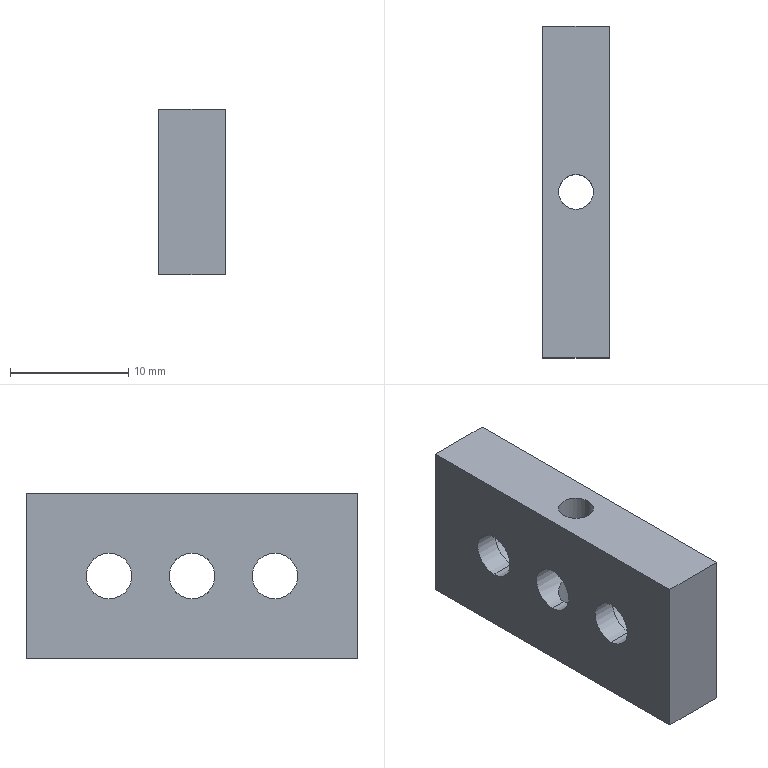Part | SolidWorks | features SplitBody 1 | 1 solid | 22 faces | box 5.6 x 28 x 14 mm | volume 1741 mm3 | cylinder 14 | plane 8 | commonest cylinder face diameters 3.85 x6 2.94 x4 7 x4
STEP:
#1=CARTESIAN_POINT('',(475.805,242.859,-463.116));
#2=VERTEX_POINT('',#1);
#3=CARTESIAN_POINT('',(478.745,242.859,-463.116));
#4=VERTEX_POINT('',#3);
#5=CARTESIAN_POINT('',(477.275,242.859,-463.116));
#6=DIRECTION('',(0.,0.,1.));
#7=DIRECTION('',(1.,0.,0.));
#8=AXIS2_PLACEMENT_3D('',#5,#6,#7);
#9=CIRCLE('',#8,1.47);
#10=EDGE_CURVE('',#2,#4,#9,.T.);
#11=ORIENTED_EDGE('',*,*,#10,.F.);
#12=CARTESIAN_POINT('',(475.805,242.859,-458.041));
#13=VERTEX_POINT('',#12);
#14=CARTESIAN_POINT('',(475.805,242.859,-449.116));
#15=DIRECTION('',(0.,0.,1.));
#16=VECTOR('',#15,1000.);
#17=LINE('',#14,#16);
#18=EDGE_CURVE('',#2,#13,#17,.T.);
#19=ORIENTED_EDGE('',*,*,#18,.T.);
#20=CARTESIAN_POINT('',(478.745,242.859,-458.041));
#21=VERTEX_POINT('',#20);
#22=CARTESIAN_POINT('',(478.745,242.859,-458.041));
#23=CARTESIAN_POINT('',(478.745,242.657,-458.041));
#24=CARTESIAN_POINT('',(478.702,242.455,-458.007));
#25=CARTESIAN_POINT('',(478.548,242.098,-457.894));
#26=CARTESIAN_POINT('',(478.439,241.942,-457.815));
#27=CARTESIAN_POINT('',(478.177,241.683,-457.648));
#28=CARTESIAN_POINT('',(478.024,241.58,-457.558));
#29=CARTESIAN_POINT('',(477.764,241.47,-457.449));
#30=CARTESIAN_POINT('',(477.671,241.44,-457.416));
#31=CARTESIAN_POINT('',(477.478,241.4,-457.371));
#32=CARTESIAN_POINT('',(477.376,241.389,-457.358));
#33=CARTESIAN_POINT('',(477.174,241.389,-457.359));
#34=CARTESIAN_POINT('',(477.072,241.4,-457.371));
#35=CARTESIAN_POINT('',(476.879,241.44,-457.417));
#36=CARTESIAN_POINT('',(476.788,241.469,-457.448));
#37=CARTESIAN_POINT('',(476.526,241.58,-457.558));
#38=CARTESIAN_POINT('',(476.375,241.682,-457.647));
#39=CARTESIAN_POINT('',(476.111,241.943,-457.816));
#40=CARTESIAN_POINT('',(476.004,242.096,-457.893));
#41=CARTESIAN_POINT('',(475.887,242.365,-457.979));
#42=CARTESIAN_POINT('',(475.857,242.459,-458.001));
#43=CARTESIAN_POINT('',(475.816,242.655,-458.032));
#44=CARTESIAN_POINT('',(475.805,242.757,-458.041));
#45=CARTESIAN_POINT('',(475.805,242.859,-458.041));
#46=B_SPLINE_CURVE_WITH_KNOTS('',3,(#22,#23,#24,#25,#26,#27,#28,#29,#30,#31,#32,#33,#34,#35,#36,#37,#38,#39,#40,#41,#42,#43,#44,#45),.UNSPECIFIED.,.F.,.F.,(4,2,2,2,2,2,2,2,2,2,2,4),(0.004827,0.005429,0.006031,0.006633,0.006935,0.007236,0.007537,0.007838,0.00844,0.009042,0.009343,0.009644),.UNSPECIFIED.);
#47=EDGE_CURVE('',#21,#13,#46,.T.);
#48=ORIENTED_EDGE('',*,*,#47,.F.);
#49=CARTESIAN_POINT('',(478.745,242.859,-449.116));
#50=DIRECTION('',(0.,0.,1.));
#51=VECTOR('',#50,1000.);
#52=LINE('',#49,#51);
#53=EDGE_CURVE('',#4,#21,#52,.T.);
#54=ORIENTED_EDGE('',*,*,#53,.F.);
#55=EDGE_LOOP('',(#11,#19,#48,#54));
#56=FACE_OUTER_BOUND('',#55,.T.);
#57=CARTESIAN_POINT('',(477.275,242.859,-449.116));
#58=DIRECTION('',(0.,0.,1.));
#59=DIRECTION('',(1.,0.,0.));
#60=AXIS2_PLACEMENT_3D('',#57,#58,#59);
#61=CYLINDRICAL_SURFACE('',#60,1.47);
#62=ADVANCED_FACE('',(#56),#61,.F.);
#63=CARTESIAN_POINT('',(475.805,242.859,-454.191));
#64=VERTEX_POINT('',#63);
#65=CARTESIAN_POINT('',(478.745,242.859,-454.191));
#66=VERTEX_POINT('',#65);
#67=CARTESIAN_POINT('',(475.805,242.859,-454.191));
#68=CARTESIAN_POINT('',(475.805,242.657,-454.191));
#69=CARTESIAN_POINT('',(475.849,242.455,-454.224));
#70=CARTESIAN_POINT('',(476.003,242.098,-454.337));
#71=CARTESIAN_POINT('',(476.112,241.942,-454.416));
#72=CARTESIAN_POINT('',(476.374,241.683,-454.584));
#73=CARTESIAN_POINT('',(476.527,241.58,-454.673));
#74=CARTESIAN_POINT('',(476.787,241.47,-454.782));
#75=CARTESIAN_POINT('',(476.88,241.44,-454.815));
#76=CARTESIAN_POINT('',(477.073,241.4,-454.86));
#77=CARTESIAN_POINT('',(477.175,241.389,-454.873));
#78=CARTESIAN_POINT('',(477.377,241.389,-454.873));
#79=CARTESIAN_POINT('',(477.478,241.4,-454.86));
#80=CARTESIAN_POINT('',(477.672,241.44,-454.814));
#81=CARTESIAN_POINT('',(477.763,241.469,-454.783));
#82=CARTESIAN_POINT('',(478.025,241.58,-454.673));
#83=CARTESIAN_POINT('',(478.176,241.682,-454.584));
#84=CARTESIAN_POINT('',(478.44,241.943,-454.415));
#85=CARTESIAN_POINT('',(478.547,242.096,-454.338));
#86=CARTESIAN_POINT('',(478.663,242.365,-454.253));
#87=CARTESIAN_POINT('',(478.693,242.459,-454.23));
#88=CARTESIAN_POINT('',(478.734,242.655,-454.199));
#89=CARTESIAN_POINT('',(478.745,242.757,-454.191));
#90=CARTESIAN_POINT('',(478.745,242.859,-454.191));
#91=B_SPLINE_CURVE_WITH_KNOTS('',3,(#67,#68,#69,#70,#71,#72,#73,#74,#75,#76,#77,#78,#79,#80,#81,#82,#83,#84,#85,#86,#87,#88,#89,#90),.UNSPECIFIED.,.F.,.F.,(4,2,2,2,2,2,2,2,2,2,2,4),(0.004827,0.005429,0.006031,0.006633,0.006935,0.007236,0.007537,0.007838,0.00844,0.009042,0.009343,0.009644),.UNSPECIFIED.);
#92=EDGE_CURVE('',#64,#66,#91,.T.);
#93=ORIENTED_EDGE('',*,*,#92,.F.);
#94=CARTESIAN_POINT('',(475.805,242.859,-449.116));
#95=VERTEX_POINT('',#94);
#96=CARTESIAN_POINT('',(475.805,242.859,-449.116));
#97=DIRECTION('',(0.,0.,1.));
#98=VECTOR('',#97,1000.);
#99=LINE('',#96,#98);
#100=EDGE_CURVE('',#64,#95,#99,.T.);
#101=ORIENTED_EDGE('',*,*,#100,.T.);
#102=CARTESIAN_POINT('',(478.745,242.859,-449.116));
#103=VERTEX_POINT('',#102);
#104=CARTESIAN_POINT('',(477.275,242.859,-449.116));
#105=DIRECTION('',(0.,0.,1.));
#106=DIRECTION('',(1.,0.,0.));
#107=AXIS2_PLACEMENT_3D('',#104,#105,#106);
#108=CIRCLE('',#107,1.47);
#109=EDGE_CURVE('',#95,#103,#108,.T.);
#110=ORIENTED_EDGE('',*,*,#109,.T.);
#111=CARTESIAN_POINT('',(478.745,242.859,-449.116));
#112=DIRECTION('',(0.,0.,1.));
#113=VECTOR('',#112,1000.);
#114=LINE('',#111,#113);
#115=EDGE_CURVE('',#66,#103,#114,.T.);
#116=ORIENTED_EDGE('',*,*,#115,.F.);
#117=EDGE_LOOP('',(#93,#101,#110,#116));
#118=FACE_OUTER_BOUND('',#117,.T.);
#119=CARTESIAN_POINT('',(477.275,242.859,-449.116));
#120=DIRECTION('',(0.,0.,1.));
#121=DIRECTION('',(1.,0.,0.));
#122=AXIS2_PLACEMENT_3D('',#119,#120,#121);
#123=CYLINDRICAL_SURFACE('',#122,1.47);
#124=ADVANCED_FACE('',(#118),#123,.F.);
#125=CARTESIAN_POINT('',(474.475,242.859,-454.191));
#126=VERTEX_POINT('',#125);
#127=CARTESIAN_POINT('',(474.475,242.859,-458.041));
#128=VERTEX_POINT('',#127);
#129=CARTESIAN_POINT('',(474.475,242.859,-456.116));
#130=DIRECTION('',(1.,0.,0.));
#131=DIRECTION('',(0.,0.,-1.));
#132=AXIS2_PLACEMENT_3D('',#129,#130,#131);
#133=CIRCLE('',#132,1.925);
#134=EDGE_CURVE('',#126,#128,#133,.T.);
#135=ORIENTED_EDGE('',*,*,#134,.F.);
#136=CARTESIAN_POINT('',(474.475,242.859,-454.191));
#137=DIRECTION('',(1.,0.,0.));
#138=VECTOR('',#137,1000.);
#139=LINE('',#136,#138);
#140=EDGE_CURVE('',#126,#64,#139,.T.);
#141=ORIENTED_EDGE('',*,*,#140,.T.);
#142=ORIENTED_EDGE('',*,*,#92,.T.);
#143=CARTESIAN_POINT('',(480.075,242.859,-454.191));
#144=VERTEX_POINT('',#143);
#145=CARTESIAN_POINT('',(474.475,242.859,-454.191));
#146=DIRECTION('',(1.,0.,0.));
#147=VECTOR('',#146,1000.);
#148=LINE('',#145,#147);
#149=EDGE_CURVE('',#66,#144,#148,.T.);
#150=ORIENTED_EDGE('',*,*,#149,.T.);
#151=CARTESIAN_POINT('',(480.075,242.859,-458.041));
#152=VERTEX_POINT('',#151);
#153=CARTESIAN_POINT('',(480.075,242.859,-456.116));
#154=DIRECTION('',(1.,0.,0.));
#155=DIRECTION('',(0.,0.,-1.));
#156=AXIS2_PLACEMENT_3D('',#153,#154,#155);
#157=CIRCLE('',#156,1.925);
#158=EDGE_CURVE('',#144,#152,#157,.T.);
#159=ORIENTED_EDGE('',*,*,#158,.T.);
#160=CARTESIAN_POINT('',(474.475,242.859,-458.041));
#161=DIRECTION('',(1.,0.,0.));
#162=VECTOR('',#161,1000.);
#163=LINE('',#160,#162);
#164=EDGE_CURVE('',#21,#152,#163,.T.);
#165=ORIENTED_EDGE('',*,*,#164,.F.);
#166=ORIENTED_EDGE('',*,*,#47,.T.);
#167=CARTESIAN_POINT('',(474.475,242.859,-458.041));
#168=DIRECTION('',(1.,0.,0.));
#169=VECTOR('',#168,1000.);
#170=LINE('',#167,#169);
#171=EDGE_CURVE('',#128,#13,#170,.T.);
#172=ORIENTED_EDGE('',*,*,#171,.F.);
#173=EDGE_LOOP('',(#135,#141,#142,#150,#159,#165,#166,#172));
#174=FACE_OUTER_BOUND('',#173,.T.);
#175=CARTESIAN_POINT('',(474.475,242.859,-456.116));
#176=DIRECTION('',(1.,0.,0.));
#177=DIRECTION('',(0.,0.,-1.));
#178=AXIS2_PLACEMENT_3D('',#175,#176,#177);
#179=CYLINDRICAL_SURFACE('',#178,1.925);
#180=ADVANCED_FACE('',(#174),#179,.F.);
#181=CARTESIAN_POINT('',(476.575,249.859,-452.616));
#182=VERTEX_POINT('',#181);
#183=CARTESIAN_POINT('',(476.575,249.859,-459.616));
#184=VERTEX_POINT('',#183);
#185=CARTESIAN_POINT('',(476.575,249.859,-456.116));
#186=DIRECTION('',(1.,0.,0.));
#187=DIRECTION('',(0.,0.,-1.));
#188=AXIS2_PLACEMENT_3D('',#185,#186,#187);
#189=CIRCLE('',#188,3.5);
#190=EDGE_CURVE('',#182,#184,#189,.T.);
#191=ORIENTED_EDGE('',*,*,#190,.F.);
#192=CARTESIAN_POINT('',(480.075,249.859,-452.616));
#193=VERTEX_POINT('',#192);
#194=CARTESIAN_POINT('',(480.075,249.859,-452.616));
#195=DIRECTION('',(1.,0.,0.));
#196=VECTOR('',#195,1000.);
#197=LINE('',#194,#196);
#198=EDGE_CURVE('',#182,#193,#197,.T.);
#199=ORIENTED_EDGE('',*,*,#198,.T.);
#200=CARTESIAN_POINT('',(480.075,249.859,-459.616));
#201=VERTEX_POINT('',#200);
#202=CARTESIAN_POINT('',(480.075,249.859,-456.116));
#203=DIRECTION('',(1.,0.,0.));
#204=DIRECTION('',(0.,0.,-1.));
#205=AXIS2_PLACEMENT_3D('',#202,#203,#204);
#206=CIRCLE('',#205,3.5);
#207=EDGE_CURVE('',#193,#201,#206,.T.);
#208=ORIENTED_EDGE('',*,*,#207,.T.);
#209=CARTESIAN_POINT('',(480.075,249.859,-459.616));
#210=DIRECTION('',(1.,0.,0.));
#211=VECTOR('',#210,1000.);
#212=LINE('',#209,#211);
#213=EDGE_CURVE('',#184,#201,#212,.T.);
#214=ORIENTED_EDGE('',*,*,#213,.F.);
#215=EDGE_LOOP('',(#191,#199,#208,#214));
#216=FACE_OUTER_BOUND('',#215,.T.);
#217=CARTESIAN_POINT('',(480.075,249.859,-456.116));
#218=DIRECTION('',(1.,0.,0.));
#219=DIRECTION('',(0.,0.,-1.));
#220=AXIS2_PLACEMENT_3D('',#217,#218,#219);
#221=CYLINDRICAL_SURFACE('',#220,3.5);
#222=ADVANCED_FACE('',(#216),#221,.F.);
#223=CARTESIAN_POINT('',(474.475,249.859,-454.191));
#224=VERTEX_POINT('',#223);
#225=CARTESIAN_POINT('',(474.475,249.859,-458.041));
#226=VERTEX_POINT('',#225);
#227=CARTESIAN_POINT('',(474.475,249.859,-456.116));
#228=DIRECTION('',(1.,0.,0.));
#229=DIRECTION('',(0.,0.,-1.));
#230=AXIS2_PLACEMENT_3D('',#227,#228,#229);
#231=CIRCLE('',#230,1.925);
#232=EDGE_CURVE('',#224,#226,#231,.T.);
#233=ORIENTED_EDGE('',*,*,#232,.F.);
#234=CARTESIAN_POINT('',(476.575,249.859,-454.191));
#235=VERTEX_POINT('',#234);
#236=CARTESIAN_POINT('',(480.075,249.859,-454.191));
#237=DIRECTION('',(1.,0.,0.));
#238=VECTOR('',#237,1000.);
#239=LINE('',#236,#238);
#240=EDGE_CURVE('',#224,#235,#239,.T.);
#241=ORIENTED_EDGE('',*,*,#240,.T.);
#242=CARTESIAN_POINT('',(476.575,249.859,-458.041));
#243=VERTEX_POINT('',#242);
#244=CARTESIAN_POINT('',(476.575,249.859,-456.116));
#245=DIRECTION('',(1.,0.,0.));
#246=DIRECTION('',(0.,0.,-1.));
#247=AXIS2_PLACEMENT_3D('',#244,#245,#246);
#248=CIRCLE('',#247,1.925);
#249=EDGE_CURVE('',#235,#243,#248,.T.);
#250=ORIENTED_EDGE('',*,*,#249,.T.);
#251=CARTESIAN_POINT('',(480.075,249.859,-458.041));
#252=DIRECTION('',(1.,0.,0.));
#253=VECTOR('',#252,1000.);
#254=LINE('',#251,#253);
#255=EDGE_CURVE('',#226,#243,#254,.T.);
#256=ORIENTED_EDGE('',*,*,#255,.F.);
#257=EDGE_LOOP('',(#233,#241,#250,#256));
#258=FACE_OUTER_BOUND('',#257,.T.);
#259=CARTESIAN_POINT('',(480.075,249.859,-456.116));
#260=DIRECTION('',(1.,0.,0.));
#261=DIRECTION('',(0.,0.,-1.));
#262=AXIS2_PLACEMENT_3D('',#259,#260,#261);
#263=CYLINDRICAL_SURFACE('',#262,1.925);
#264=ADVANCED_FACE('',(#258),#263,.F.);
#265=CARTESIAN_POINT('',(476.575,235.859,-452.616));
#266=VERTEX_POINT('',#265);
#267=CARTESIAN_POINT('',(476.575,235.859,-459.616));
#268=VERTEX_POINT('',#267);
#269=CARTESIAN_POINT('',(476.575,235.859,-456.116));
#270=DIRECTION('',(1.,0.,0.));
#271=DIRECTION('',(0.,0.,-1.));
#272=AXIS2_PLACEMENT_3D('',#269,#270,#271);
#273=CIRCLE('',#272,3.5);
#274=EDGE_CURVE('',#266,#268,#273,.T.);
#275=ORIENTED_EDGE('',*,*,#274,.F.);
#276=CARTESIAN_POINT('',(480.075,235.859,-452.616));
#277=VERTEX_POINT('',#276);
#278=CARTESIAN_POINT('',(480.075,235.859,-452.616));
#279=DIRECTION('',(1.,0.,0.));
#280=VECTOR('',#279,1000.);
#281=LINE('',#278,#280);
#282=EDGE_CURVE('',#266,#277,#281,.T.);
#283=ORIENTED_EDGE('',*,*,#282,.T.);
#284=CARTESIAN_POINT('',(480.075,235.859,-459.616));
#285=VERTEX_POINT('',#284);
#286=CARTESIAN_POINT('',(480.075,235.859,-456.116));
#287=DIRECTION('',(1.,0.,0.));
#288=DIRECTION('',(0.,0.,-1.));
#289=AXIS2_PLACEMENT_3D('',#286,#287,#288);
#290=CIRCLE('',#289,3.5);
#291=EDGE_CURVE('',#277,#285,#290,.T.);
#292=ORIENTED_EDGE('',*,*,#291,.T.);
#293=CARTESIAN_POINT('',(480.075,235.859,-459.616));
#294=DIRECTION('',(1.,0.,0.));
#295=VECTOR('',#294,1000.);
#296=LINE('',#293,#295);
#297=EDGE_CURVE('',#268,#285,#296,.T.);
#298=ORIENTED_EDGE('',*,*,#297,.F.);
#299=EDGE_LOOP('',(#275,#283,#292,#298));
#300=FACE_OUTER_BOUND('',#299,.T.);
#301=CARTESIAN_POINT('',(480.075,235.859,-456.116));
#302=DIRECTION('',(1.,0.,0.));
#303=DIRECTION('',(0.,0.,-1.));
#304=AXIS2_PLACEMENT_3D('',#301,#302,#303);
#305=CYLINDRICAL_SURFACE('',#304,3.5);
#306=ADVANCED_FACE('',(#300),#305,.F.);
#307=CARTESIAN_POINT('',(474.475,235.859,-454.191));
#308=VERTEX_POINT('',#307);
#309=CARTESIAN_POINT('',(474.475,235.859,-458.041));
#310=VERTEX_POINT('',#309);
#311=CARTESIAN_POINT('',(474.475,235.859,-456.116));
#312=DIRECTION('',(1.,0.,0.));
#313=DIRECTION('',(0.,0.,-1.));
#314=AXIS2_PLACEMENT_3D('',#311,#312,#313);
#315=CIRCLE('',#314,1.925);
#316=EDGE_CURVE('',#308,#310,#315,.T.);
#317=ORIENTED_EDGE('',*,*,#316,.F.);
#318=CARTESIAN_POINT('',(476.575,235.859,-454.191));
#319=VERTEX_POINT('',#318);
#320=CARTESIAN_POINT('',(480.075,235.859,-454.191));
#321=DIRECTION('',(1.,0.,0.));
#322=VECTOR('',#321,1000.);
#323=LINE('',#320,#322);
#324=EDGE_CURVE('',#308,#319,#323,.T.);
#325=ORIENTED_EDGE('',*,*,#324,.T.);
#326=CARTESIAN_POINT('',(476.575,235.859,-458.041));
#327=VERTEX_POINT('',#326);
#328=CARTESIAN_POINT('',(476.575,235.859,-456.116));
#329=DIRECTION('',(1.,0.,0.));
#330=DIRECTION('',(0.,0.,-1.));
#331=AXIS2_PLACEMENT_3D('',#328,#329,#330);
#332=CIRCLE('',#331,1.925);
#333=EDGE_CURVE('',#319,#327,#332,.T.);
#334=ORIENTED_EDGE('',*,*,#333,.T.);
#335=CARTESIAN_POINT('',(480.075,235.859,-458.041));
#336=DIRECTION('',(1.,0.,0.));
#337=VECTOR('',#336,1000.);
#338=LINE('',#335,#337);
#339=EDGE_CURVE('',#310,#327,#338,.T.);
#340=ORIENTED_EDGE('',*,*,#339,.F.);
#341=EDGE_LOOP('',(#317,#325,#334,#340));
#342=FACE_OUTER_BOUND('',#341,.T.);
#343=CARTESIAN_POINT('',(480.075,235.859,-456.116));
#344=DIRECTION('',(1.,0.,0.));
#345=DIRECTION('',(0.,0.,-1.));
#346=AXIS2_PLACEMENT_3D('',#343,#344,#345);
#347=CYLINDRICAL_SURFACE('',#346,1.925);
#348=ADVANCED_FACE('',(#342),#347,.F.);
#349=CARTESIAN_POINT('',(477.275,242.859,-449.116));
#350=DIRECTION('',(0.,0.,1.));
#351=DIRECTION('',(1.,0.,0.));
#352=AXIS2_PLACEMENT_3D('',#349,#350,#351);
#353=CIRCLE('',#352,1.47);
#354=EDGE_CURVE('',#103,#95,#353,.T.);
#355=ORIENTED_EDGE('',*,*,#354,.F.);
#356=ORIENTED_EDGE('',*,*,#109,.F.);
#357=EDGE_LOOP('',(#355,#356));
#358=FACE_BOUND('',#357,.T.);
#359=CARTESIAN_POINT('',(474.475,256.859,-449.116));
#360=VERTEX_POINT('',#359);
#361=CARTESIAN_POINT('',(474.475,228.859,-449.116));
#362=VERTEX_POINT('',#361);
#363=CARTESIAN_POINT('',(474.475,256.859,-449.116));
#364=DIRECTION('',(0.,-1.,0.));
#365=VECTOR('',#364,1000.);
#366=LINE('',#363,#365);
#367=EDGE_CURVE('',#360,#362,#366,.T.);
#368=ORIENTED_EDGE('',*,*,#367,.T.);
#369=CARTESIAN_POINT('',(480.075,228.859,-449.116));
#370=VERTEX_POINT('',#369);
#371=CARTESIAN_POINT('',(480.075,228.859,-449.116));
#372=DIRECTION('',(-1.,0.,0.));
#373=VECTOR('',#372,1000.);
#374=LINE('',#371,#373);
#375=EDGE_CURVE('',#370,#362,#374,.T.);
#376=ORIENTED_EDGE('',*,*,#375,.F.);
#377=CARTESIAN_POINT('',(480.075,256.859,-449.116));
#378=VERTEX_POINT('',#377);
#379=CARTESIAN_POINT('',(480.075,256.859,-449.116));
#380=DIRECTION('',(0.,-1.,0.));
#381=VECTOR('',#380,1000.);
#382=LINE('',#379,#381);
#383=EDGE_CURVE('',#378,#370,#382,.T.);
#384=ORIENTED_EDGE('',*,*,#383,.F.);
#385=CARTESIAN_POINT('',(480.075,256.859,-449.116));
#386=DIRECTION('',(-1.,0.,0.));
#387=VECTOR('',#386,1000.);
#388=LINE('',#385,#387);
#389=EDGE_CURVE('',#378,#360,#388,.T.);
#390=ORIENTED_EDGE('',*,*,#389,.T.);
#391=EDGE_LOOP('',(#368,#376,#384,#390));
#392=FACE_OUTER_BOUND('',#391,.T.);
#393=CARTESIAN_POINT('',(480.075,256.859,-449.116));
#394=DIRECTION('',(0.,0.,-1.));
#395=DIRECTION('',(0.,1.,0.));
#396=AXIS2_PLACEMENT_3D('',#393,#394,#395);
#397=PLANE('',#396);
#398=ADVANCED_FACE('',(#358,#392),#397,.F.);
#399=CARTESIAN_POINT('',(474.475,228.859,-463.116));
#400=VERTEX_POINT('',#399);
#401=CARTESIAN_POINT('',(474.475,228.859,-449.116));
#402=DIRECTION('',(0.,0.,-1.));
#403=VECTOR('',#402,1000.);
#404=LINE('',#401,#403);
#405=EDGE_CURVE('',#362,#400,#404,.T.);
#406=ORIENTED_EDGE('',*,*,#405,.T.);
#407=CARTESIAN_POINT('',(480.075,228.859,-463.116));
#408=VERTEX_POINT('',#407);
#409=CARTESIAN_POINT('',(480.075,228.859,-463.116));
#410=DIRECTION('',(-1.,0.,0.));
#411=VECTOR('',#410,1000.);
#412=LINE('',#409,#411);
#413=EDGE_CURVE('',#408,#400,#412,.T.);
#414=ORIENTED_EDGE('',*,*,#413,.F.);
#415=CARTESIAN_POINT('',(480.075,228.859,-449.116));
#416=DIRECTION('',(0.,0.,-1.));
#417=VECTOR('',#416,1000.);
#418=LINE('',#415,#417);
#419=EDGE_CURVE('',#370,#408,#418,.T.);
#420=ORIENTED_EDGE('',*,*,#419,.F.);
#421=ORIENTED_EDGE('',*,*,#375,.T.);
#422=EDGE_LOOP('',(#406,#414,#420,#421));
#423=FACE_OUTER_BOUND('',#422,.T.);
#424=CARTESIAN_POINT('',(480.075,228.859,-449.116));
#425=DIRECTION('',(0.,1.,0.));
#426=DIRECTION('',(1.,0.,0.));
#427=AXIS2_PLACEMENT_3D('',#424,#425,#426);
#428=PLANE('',#427);
#429=ADVANCED_FACE('',(#423),#428,.F.);
#430=CARTESIAN_POINT('',(477.275,242.859,-463.116));
#431=DIRECTION('',(0.,0.,1.));
#432=DIRECTION('',(1.,0.,0.));
#433=AXIS2_PLACEMENT_3D('',#430,#431,#432);
#434=CIRCLE('',#433,1.47);
#435=EDGE_CURVE('',#4,#2,#434,.T.);
#436=ORIENTED_EDGE('',*,*,#435,.T.);
#437=ORIENTED_EDGE('',*,*,#10,.T.);
#438=EDGE_LOOP('',(#436,#437));
#439=FACE_BOUND('',#438,.T.);
#440=CARTESIAN_POINT('',(474.475,256.859,-463.116));
#441=VERTEX_POINT('',#440);
#442=CARTESIAN_POINT('',(474.475,256.859,-463.116));
#443=DIRECTION('',(0.,1.,0.));
#444=VECTOR('',#443,1000.);
#445=LINE('',#442,#444);
#446=EDGE_CURVE('',#400,#441,#445,.T.);
#447=ORIENTED_EDGE('',*,*,#446,.T.);
#448=CARTESIAN_POINT('',(480.075,256.859,-463.116));
#449=VERTEX_POINT('',#448);
#450=CARTESIAN_POINT('',(480.075,256.859,-463.116));
#451=DIRECTION('',(-1.,0.,0.));
#452=VECTOR('',#451,1000.);
#453=LINE('',#450,#452);
#454=EDGE_CURVE('',#449,#441,#453,.T.);
#455=ORIENTED_EDGE('',*,*,#454,.F.);
#456=CARTESIAN_POINT('',(480.075,256.859,-463.116));
#457=DIRECTION('',(0.,1.,0.));
#458=VECTOR('',#457,1000.);
#459=LINE('',#456,#458);
#460=EDGE_CURVE('',#408,#449,#459,.T.);
#461=ORIENTED_EDGE('',*,*,#460,.F.);
#462=ORIENTED_EDGE('',*,*,#413,.T.);
#463=EDGE_LOOP('',(#447,#455,#461,#462));
#464=FACE_OUTER_BOUND('',#463,.T.);
#465=CARTESIAN_POINT('',(480.075,256.859,-463.116));
#466=DIRECTION('',(0.,0.,1.));
#467=DIRECTION('',(1.,0.,0.));
#468=AXIS2_PLACEMENT_3D('',#465,#466,#467);
#469=PLANE('',#468);
#470=ADVANCED_FACE('',(#439,#464),#469,.F.);
#471=CARTESIAN_POINT('',(474.475,256.859,-449.116));
#472=DIRECTION('',(0.,0.,1.));
#473=VECTOR('',#472,1000.);
#474=LINE('',#471,#473);
#475=EDGE_CURVE('',#441,#360,#474,.T.);
#476=ORIENTED_EDGE('',*,*,#475,.T.);
#477=ORIENTED_EDGE('',*,*,#389,.F.);
#478=CARTESIAN_POINT('',(480.075,256.859,-449.116));
#479=DIRECTION('',(0.,0.,1.));
#480=VECTOR('',#479,1000.);
#481=LINE('',#478,#480);
#482=EDGE_CURVE('',#449,#378,#481,.T.);
#483=ORIENTED_EDGE('',*,*,#482,.F.);
#484=ORIENTED_EDGE('',*,*,#454,.T.);
#485=EDGE_LOOP('',(#476,#477,#483,#484));
#486=FACE_OUTER_BOUND('',#485,.T.);
#487=CARTESIAN_POINT('',(480.075,256.859,-449.116));
#488=DIRECTION('',(0.,-1.,0.));
#489=DIRECTION('',(-1.,0.,0.));
#490=AXIS2_PLACEMENT_3D('',#487,#488,#489);
#491=PLANE('',#490);
#492=ADVANCED_FACE('',(#486),#491,.F.);
#493=CARTESIAN_POINT('',(480.075,242.859,-456.116));
#494=DIRECTION('',(1.,0.,0.));
#495=DIRECTION('',(0.,0.,-1.));
#496=AXIS2_PLACEMENT_3D('',#493,#494,#495);
#497=CIRCLE('',#496,1.925);
#498=EDGE_CURVE('',#152,#144,#497,.T.);
#499=ORIENTED_EDGE('',*,*,#498,.F.);
#500=ORIENTED_EDGE('',*,*,#158,.F.);
#501=EDGE_LOOP('',(#499,#500));
#502=FACE_BOUND('',#501,.T.);
#503=CARTESIAN_POINT('',(480.075,249.859,-456.116));
#504=DIRECTION('',(1.,0.,0.));
#505=DIRECTION('',(0.,0.,-1.));
#506=AXIS2_PLACEMENT_3D('',#503,#504,#505);
#507=CIRCLE('',#506,3.5);
#508=EDGE_CURVE('',#201,#193,#507,.T.);
#509=ORIENTED_EDGE('',*,*,#508,.F.);
#510=ORIENTED_EDGE('',*,*,#207,.F.);
#511=EDGE_LOOP('',(#509,#510));
#512=FACE_BOUND('',#511,.T.);
#513=CARTESIAN_POINT('',(480.075,235.859,-456.116));
#514=DIRECTION('',(1.,0.,0.));
#515=DIRECTION('',(0.,0.,-1.));
#516=AXIS2_PLACEMENT_3D('',#513,#514,#515);
#517=CIRCLE('',#516,3.5);
#518=EDGE_CURVE('',#285,#277,#517,.T.);
#519=ORIENTED_EDGE('',*,*,#518,.F.);
#520=ORIENTED_EDGE('',*,*,#291,.F.);
#521=EDGE_LOOP('',(#519,#520));
#522=FACE_BOUND('',#521,.T.);
#523=ORIENTED_EDGE('',*,*,#383,.T.);
#524=ORIENTED_EDGE('',*,*,#419,.T.);
#525=ORIENTED_EDGE('',*,*,#460,.T.);
#526=ORIENTED_EDGE('',*,*,#482,.T.);
#527=EDGE_LOOP('',(#523,#524,#525,#526));
#528=FACE_OUTER_BOUND('',#527,.T.);
#529=CARTESIAN_POINT('',(480.075,228.859,-449.116));
#530=DIRECTION('',(1.,0.,0.));
#531=DIRECTION('',(0.,0.,-1.));
#532=AXIS2_PLACEMENT_3D('',#529,#530,#531);
#533=PLANE('',#532);
#534=ADVANCED_FACE('',(#502,#512,#522,#528),#533,.T.);
#535=CARTESIAN_POINT('',(474.475,242.859,-456.116));
#536=DIRECTION('',(1.,0.,0.));
#537=DIRECTION('',(0.,0.,-1.));
#538=AXIS2_PLACEMENT_3D('',#535,#536,#537);
#539=CIRCLE('',#538,1.925);
#540=EDGE_CURVE('',#128,#126,#539,.T.);
#541=ORIENTED_EDGE('',*,*,#540,.T.);
#542=ORIENTED_EDGE('',*,*,#134,.T.);
#543=EDGE_LOOP('',(#541,#542));
#544=FACE_BOUND('',#543,.T.);
#545=CARTESIAN_POINT('',(474.475,249.859,-456.116));
#546=DIRECTION('',(1.,0.,0.));
#547=DIRECTION('',(0.,0.,-1.));
#548=AXIS2_PLACEMENT_3D('',#545,#546,#547);
#549=CIRCLE('',#548,1.925);
#550=EDGE_CURVE('',#226,#224,#549,.T.);
#551=ORIENTED_EDGE('',*,*,#550,.T.);
#552=ORIENTED_EDGE('',*,*,#232,.T.);
#553=EDGE_LOOP('',(#551,#552));
#554=FACE_BOUND('',#553,.T.);
#555=CARTESIAN_POINT('',(474.475,235.859,-456.116));
#556=DIRECTION('',(1.,0.,0.));
#557=DIRECTION('',(0.,0.,-1.));
#558=AXIS2_PLACEMENT_3D('',#555,#556,#557);
#559=CIRCLE('',#558,1.925);
#560=EDGE_CURVE('',#310,#308,#559,.T.);
#561=ORIENTED_EDGE('',*,*,#560,.T.);
#562=ORIENTED_EDGE('',*,*,#316,.T.);
#563=EDGE_LOOP('',(#561,#562));
#564=FACE_BOUND('',#563,.T.);
#565=ORIENTED_EDGE('',*,*,#367,.F.);
#566=ORIENTED_EDGE('',*,*,#475,.F.);
#567=ORIENTED_EDGE('',*,*,#446,.F.);
#568=ORIENTED_EDGE('',*,*,#405,.F.);
#569=EDGE_LOOP('',(#565,#566,#567,#568));
#570=FACE_OUTER_BOUND('',#569,.T.);
#571=CARTESIAN_POINT('',(474.475,228.859,-449.116));
#572=DIRECTION('',(1.,0.,0.));
#573=DIRECTION('',(0.,0.,-1.));
#574=AXIS2_PLACEMENT_3D('',#571,#572,#573);
#575=PLANE('',#574);
#576=ADVANCED_FACE('',(#544,#554,#564,#570),#575,.F.);
#577=ORIENTED_EDGE('',*,*,#324,.F.);
#578=ORIENTED_EDGE('',*,*,#560,.F.);
#579=ORIENTED_EDGE('',*,*,#339,.T.);
#580=CARTESIAN_POINT('',(476.575,235.859,-456.116));
#581=DIRECTION('',(1.,0.,0.));
#582=DIRECTION('',(0.,0.,-1.));
#583=AXIS2_PLACEMENT_3D('',#580,#581,#582);
#584=CIRCLE('',#583,1.925);
#585=EDGE_CURVE('',#327,#319,#584,.T.);
#586=ORIENTED_EDGE('',*,*,#585,.T.);
#587=EDGE_LOOP('',(#577,#578,#579,#586));
#588=FACE_OUTER_BOUND('',#587,.T.);
#589=CARTESIAN_POINT('',(480.075,235.859,-456.116));
#590=DIRECTION('',(1.,0.,0.));
#591=DIRECTION('',(0.,0.,-1.));
#592=AXIS2_PLACEMENT_3D('',#589,#590,#591);
#593=CYLINDRICAL_SURFACE('',#592,1.925);
#594=ADVANCED_FACE('',(#588),#593,.F.);
#595=ORIENTED_EDGE('',*,*,#585,.F.);
#596=ORIENTED_EDGE('',*,*,#333,.F.);
#597=EDGE_LOOP('',(#595,#596));
#598=FACE_BOUND('',#597,.T.);
#599=CARTESIAN_POINT('',(476.575,235.859,-456.116));
#600=DIRECTION('',(1.,0.,0.));
#601=DIRECTION('',(0.,0.,-1.));
#602=AXIS2_PLACEMENT_3D('',#599,#600,#601);
#603=CIRCLE('',#602,3.5);
#604=EDGE_CURVE('',#268,#266,#603,.T.);
#605=ORIENTED_EDGE('',*,*,#604,.T.);
#606=ORIENTED_EDGE('',*,*,#274,.T.);
#607=EDGE_LOOP('',(#605,#606));
#608=FACE_OUTER_BOUND('',#607,.T.);
#609=CARTESIAN_POINT('',(476.575,235.859,-458.041));
#610=DIRECTION('',(-1.,0.,0.));
#611=DIRECTION('',(0.,0.,1.));
#612=AXIS2_PLACEMENT_3D('',#609,#610,#611);
#613=PLANE('',#612);
#614=ADVANCED_FACE('',(#598,#608),#613,.F.);
#615=ORIENTED_EDGE('',*,*,#282,.F.);
#616=ORIENTED_EDGE('',*,*,#604,.F.);
#617=ORIENTED_EDGE('',*,*,#297,.T.);
#618=ORIENTED_EDGE('',*,*,#518,.T.);
#619=EDGE_LOOP('',(#615,#616,#617,#618));
#620=FACE_OUTER_BOUND('',#619,.T.);
#621=CARTESIAN_POINT('',(480.075,235.859,-456.116));
#622=DIRECTION('',(1.,0.,0.));
#623=DIRECTION('',(0.,0.,-1.));
#624=AXIS2_PLACEMENT_3D('',#621,#622,#623);
#625=CYLINDRICAL_SURFACE('',#624,3.5);
#626=ADVANCED_FACE('',(#620),#625,.F.);
#627=ORIENTED_EDGE('',*,*,#240,.F.);
#628=ORIENTED_EDGE('',*,*,#550,.F.);
#629=ORIENTED_EDGE('',*,*,#255,.T.);
#630=CARTESIAN_POINT('',(476.575,249.859,-456.116));
#631=DIRECTION('',(1.,0.,0.));
#632=DIRECTION('',(0.,0.,-1.));
#633=AXIS2_PLACEMENT_3D('',#630,#631,#632);
#634=CIRCLE('',#633,1.925);
#635=EDGE_CURVE('',#243,#235,#634,.T.);
#636=ORIENTED_EDGE('',*,*,#635,.T.);
#637=EDGE_LOOP('',(#627,#628,#629,#636));
#638=FACE_OUTER_BOUND('',#637,.T.);
#639=CARTESIAN_POINT('',(480.075,249.859,-456.116));
#640=DIRECTION('',(1.,0.,0.));
#641=DIRECTION('',(0.,0.,-1.));
#642=AXIS2_PLACEMENT_3D('',#639,#640,#641);
#643=CYLINDRICAL_SURFACE('',#642,1.925);
#644=ADVANCED_FACE('',(#638),#643,.F.);
#645=ORIENTED_EDGE('',*,*,#635,.F.);
#646=ORIENTED_EDGE('',*,*,#249,.F.);
#647=EDGE_LOOP('',(#645,#646));
#648=FACE_BOUND('',#647,.T.);
#649=CARTESIAN_POINT('',(476.575,249.859,-456.116));
#650=DIRECTION('',(1.,0.,0.));
#651=DIRECTION('',(0.,0.,-1.));
#652=AXIS2_PLACEMENT_3D('',#649,#650,#651);
#653=CIRCLE('',#652,3.5);
#654=EDGE_CURVE('',#184,#182,#653,.T.);
#655=ORIENTED_EDGE('',*,*,#654,.T.);
#656=ORIENTED_EDGE('',*,*,#190,.T.);
#657=EDGE_LOOP('',(#655,#656));
#658=FACE_OUTER_BOUND('',#657,.T.);
#659=CARTESIAN_POINT('',(476.575,249.859,-458.041));
#660=DIRECTION('',(-1.,0.,0.));
#661=DIRECTION('',(0.,0.,1.));
#662=AXIS2_PLACEMENT_3D('',#659,#660,#661);
#663=PLANE('',#662);
#664=ADVANCED_FACE('',(#648,#658),#663,.F.);
#665=ORIENTED_EDGE('',*,*,#198,.F.);
#666=ORIENTED_EDGE('',*,*,#654,.F.);
#667=ORIENTED_EDGE('',*,*,#213,.T.);
#668=ORIENTED_EDGE('',*,*,#508,.T.);
#669=EDGE_LOOP('',(#665,#666,#667,#668));
#670=FACE_OUTER_BOUND('',#669,.T.);
#671=CARTESIAN_POINT('',(480.075,249.859,-456.116));
#672=DIRECTION('',(1.,0.,0.));
#673=DIRECTION('',(0.,0.,-1.));
#674=AXIS2_PLACEMENT_3D('',#671,#672,#673);
#675=CYLINDRICAL_SURFACE('',#674,3.5);
#676=ADVANCED_FACE('',(#670),#675,.F.);
#677=ORIENTED_EDGE('',*,*,#140,.F.);
#678=ORIENTED_EDGE('',*,*,#540,.F.);
#679=ORIENTED_EDGE('',*,*,#171,.T.);
#680=CARTESIAN_POINT('',(475.805,242.859,-458.041));
#681=CARTESIAN_POINT('',(475.805,242.961,-458.041));
#682=CARTESIAN_POINT('',(475.816,243.061,-458.033));
#683=CARTESIAN_POINT('',(475.856,243.256,-458.002));
#684=CARTESIAN_POINT('',(475.887,243.352,-457.979));
#685=CARTESIAN_POINT('',(476.002,243.619,-457.894));
#686=CARTESIAN_POINT('',(476.111,243.776,-457.815));
#687=CARTESIAN_POINT('',(476.374,244.035,-457.648));
#688=CARTESIAN_POINT('',(476.526,244.138,-457.558));
#689=CARTESIAN_POINT('',(476.787,244.249,-457.449));
#690=CARTESIAN_POINT('',(476.88,244.278,-457.417));
#691=CARTESIAN_POINT('',(477.072,244.318,-457.371));
#692=CARTESIAN_POINT('',(477.175,244.329,-457.358));
#693=CARTESIAN_POINT('',(477.376,244.329,-457.358));
#694=CARTESIAN_POINT('',(477.478,244.318,-457.371));
#695=CARTESIAN_POINT('',(477.671,244.278,-457.417));
#696=CARTESIAN_POINT('',(477.764,244.249,-457.449));
#697=CARTESIAN_POINT('',(477.938,244.174,-457.522));
#698=CARTESIAN_POINT('',(478.019,244.13,-457.563));
#699=CARTESIAN_POINT('',(478.172,244.028,-457.647));
#700=CARTESIAN_POINT('',(478.243,243.969,-457.69));
#701=CARTESIAN_POINT('',(478.374,243.84,-457.774));
#702=CARTESIAN_POINT('',(478.433,243.769,-457.814));
#703=CARTESIAN_POINT('',(478.54,243.614,-457.888));
#704=CARTESIAN_POINT('',(478.587,243.529,-457.923));
#705=CARTESIAN_POINT('',(478.664,243.352,-457.979));
#706=CARTESIAN_POINT('',(478.694,243.256,-458.002));
#707=CARTESIAN_POINT('',(478.735,243.06,-458.033));
#708=CARTESIAN_POINT('',(478.745,242.96,-458.041));
#709=CARTESIAN_POINT('',(478.745,242.859,-458.041));
#710=B_SPLINE_CURVE_WITH_KNOTS('',3,(#680,#681,#682,#683,#684,#685,#686,#687,#688,#689,#690,#691,#692,#693,#694,#695,#696,#697,#698,#699,#700,#701,#702,#703,#704,#705,#706,#707,#708,#709),.UNSPECIFIED.,.F.,.F.,(4,2,2,2,2,2,2,2,2,2,2,2,2,2,4),(0.,0.0003017,0.0006034,0.001207,0.00181,0.002112,0.002413,0.002715,0.003017,0.003319,0.00362,0.003922,0.004224,0.004525,0.004827),.UNSPECIFIED.);
#711=EDGE_CURVE('',#13,#21,#710,.T.);
#712=ORIENTED_EDGE('',*,*,#711,.T.);
#713=ORIENTED_EDGE('',*,*,#164,.T.);
#714=ORIENTED_EDGE('',*,*,#498,.T.);
#715=ORIENTED_EDGE('',*,*,#149,.F.);
#716=CARTESIAN_POINT('',(478.745,242.859,-454.191));
#717=CARTESIAN_POINT('',(478.745,242.961,-454.191));
#718=CARTESIAN_POINT('',(478.735,243.061,-454.199));
#719=CARTESIAN_POINT('',(478.694,243.256,-454.229));
#720=CARTESIAN_POINT('',(478.664,243.352,-454.252));
#721=CARTESIAN_POINT('',(478.549,243.619,-454.337));
#722=CARTESIAN_POINT('',(478.439,243.776,-454.416));
#723=CARTESIAN_POINT('',(478.177,244.035,-454.583));
#724=CARTESIAN_POINT('',(478.025,244.138,-454.673));
#725=CARTESIAN_POINT('',(477.764,244.249,-454.782));
#726=CARTESIAN_POINT('',(477.671,244.278,-454.815));
#727=CARTESIAN_POINT('',(477.478,244.318,-454.86));
#728=CARTESIAN_POINT('',(477.376,244.329,-454.873));
#729=CARTESIAN_POINT('',(477.175,244.329,-454.873));
#730=CARTESIAN_POINT('',(477.073,244.318,-454.86));
#731=CARTESIAN_POINT('',(476.879,244.278,-454.815));
#732=CARTESIAN_POINT('',(476.786,244.249,-454.782));
#733=CARTESIAN_POINT('',(476.612,244.174,-454.709));
#734=CARTESIAN_POINT('',(476.531,244.13,-454.669));
#735=CARTESIAN_POINT('',(476.379,244.028,-454.585));
#736=CARTESIAN_POINT('',(476.307,243.969,-454.541));
#737=CARTESIAN_POINT('',(476.176,243.84,-454.457));
#738=CARTESIAN_POINT('',(476.117,243.769,-454.417));
#739=CARTESIAN_POINT('',(476.01,243.614,-454.343));
#740=CARTESIAN_POINT('',(475.963,243.529,-454.309));
#741=CARTESIAN_POINT('',(475.887,243.352,-454.252));
#742=CARTESIAN_POINT('',(475.856,243.256,-454.229));
#743=CARTESIAN_POINT('',(475.816,243.06,-454.199));
#744=CARTESIAN_POINT('',(475.805,242.96,-454.191));
#745=CARTESIAN_POINT('',(475.805,242.859,-454.191));
#746=B_SPLINE_CURVE_WITH_KNOTS('',3,(#716,#717,#718,#719,#720,#721,#722,#723,#724,#725,#726,#727,#728,#729,#730,#731,#732,#733,#734,#735,#736,#737,#738,#739,#740,#741,#742,#743,#744,#745),.UNSPECIFIED.,.F.,.F.,(4,2,2,2,2,2,2,2,2,2,2,2,2,2,4),(0.,0.0003017,0.0006034,0.001207,0.00181,0.002112,0.002413,0.002715,0.003017,0.003319,0.00362,0.003922,0.004224,0.004525,0.004827),.UNSPECIFIED.);
#747=EDGE_CURVE('',#66,#64,#746,.T.);
#748=ORIENTED_EDGE('',*,*,#747,.T.);
#749=EDGE_LOOP('',(#677,#678,#679,#712,#713,#714,#715,#748));
#750=FACE_OUTER_BOUND('',#749,.T.);
#751=CARTESIAN_POINT('',(474.475,242.859,-456.116));
#752=DIRECTION('',(1.,0.,0.));
#753=DIRECTION('',(0.,0.,-1.));
#754=AXIS2_PLACEMENT_3D('',#751,#752,#753);
#755=CYLINDRICAL_SURFACE('',#754,1.925);
#756=ADVANCED_FACE('',(#750),#755,.F.);
#757=ORIENTED_EDGE('',*,*,#100,.F.);
#758=ORIENTED_EDGE('',*,*,#747,.F.);
#759=ORIENTED_EDGE('',*,*,#115,.T.);
#760=ORIENTED_EDGE('',*,*,#354,.T.);
#761=EDGE_LOOP('',(#757,#758,#759,#760));
#762=FACE_OUTER_BOUND('',#761,.T.);
#763=CARTESIAN_POINT('',(477.275,242.859,-449.116));
#764=DIRECTION('',(0.,0.,1.));
#765=DIRECTION('',(1.,0.,0.));
#766=AXIS2_PLACEMENT_3D('',#763,#764,#765);
#767=CYLINDRICAL_SURFACE('',#766,1.47);
#768=ADVANCED_FACE('',(#762),#767,.F.);
#769=ORIENTED_EDGE('',*,*,#18,.F.);
#770=ORIENTED_EDGE('',*,*,#435,.F.);
#771=ORIENTED_EDGE('',*,*,#53,.T.);
#772=ORIENTED_EDGE('',*,*,#711,.F.);
#773=EDGE_LOOP('',(#769,#770,#771,#772));
#774=FACE_OUTER_BOUND('',#773,.T.);
#775=CARTESIAN_POINT('',(477.275,242.859,-449.116));
#776=DIRECTION('',(0.,0.,1.));
#777=DIRECTION('',(1.,0.,0.));
#778=AXIS2_PLACEMENT_3D('',#775,#776,#777);
#779=CYLINDRICAL_SURFACE('',#778,1.47);
#780=ADVANCED_FACE('',(#774),#779,.F.);
#781=CLOSED_SHELL('',(#62,#124,#180,#222,#264,#306,#348,#398,#429,#470,#492,#534,#576,#594,#614,#626,#644,#664,#676,#756,#768,#780));
#782=MANIFOLD_SOLID_BREP('',#781);
#783=CARTESIAN_POINT('',(0.,0.,0.));
#784=DIRECTION('',(0.,0.,1.));
#785=DIRECTION('',(1.,0.,0.));
#786=AXIS2_PLACEMENT_3D('',#783,#784,#785);
#787=(LENGTH_UNIT()NAMED_UNIT(*)SI_UNIT(.MILLI.,.METRE.));
#788=UNCERTAINTY_MEASURE_WITH_UNIT(LENGTH_MEASURE(0.00001),#787,'','');
#789=(NAMED_UNIT(*)PLANE_ANGLE_UNIT()SI_UNIT($,.RADIAN.));
#790=(NAMED_UNIT(*)SI_UNIT($,.STERADIAN.)SOLID_ANGLE_UNIT());
#791=(GEOMETRIC_REPRESENTATION_CONTEXT(3)GLOBAL_UNCERTAINTY_ASSIGNED_CONTEXT((#788))GLOBAL_UNIT_ASSIGNED_CONTEXT((#787,#789,#790))REPRESENTATION_CONTEXT('',''));
#792=ADVANCED_BREP_SHAPE_REPRESENTATION('',(#782,#786),#791);